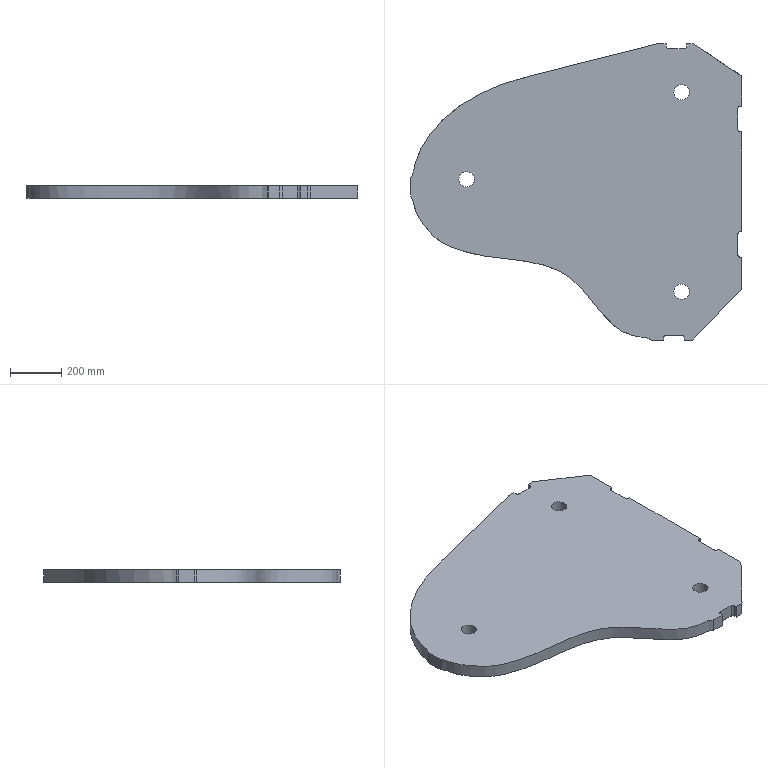Part | NX | features solid 2 | 1 solid | 45 faces | box 1295 x 1160 x 50 mm | volume 53186483 mm3 | plane 22 | spline 12 | cylinder 11 | commonest cylinder face diameters 20 x8 60 x3